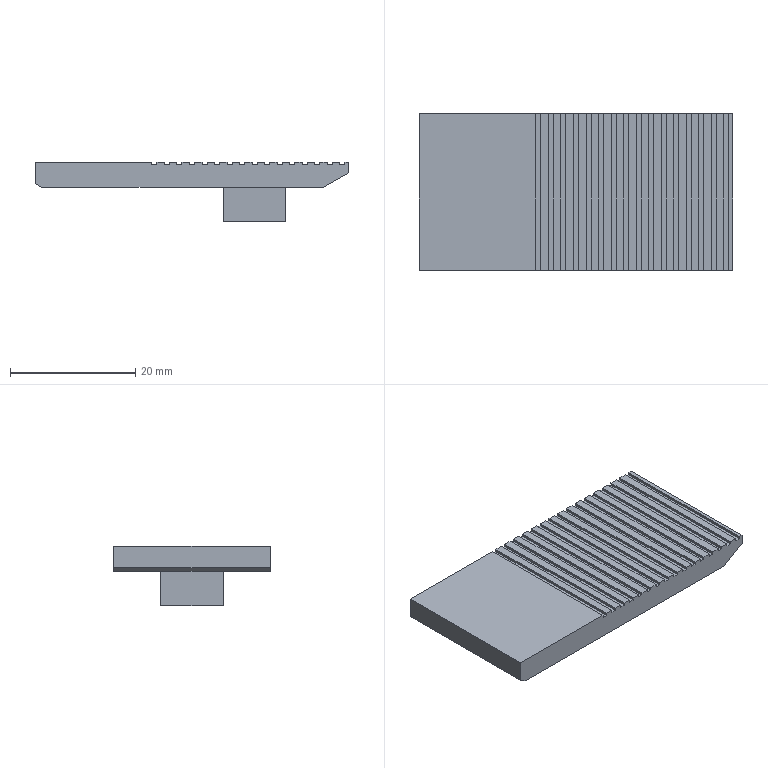Part | SolidWorks | features Chamfer 2, ICE 2, Extrusion 1, LPattern 1 | 1 solid | 77 faces | box 50 x 25 x 9.5 mm | volume 5299 mm3 | plane 77